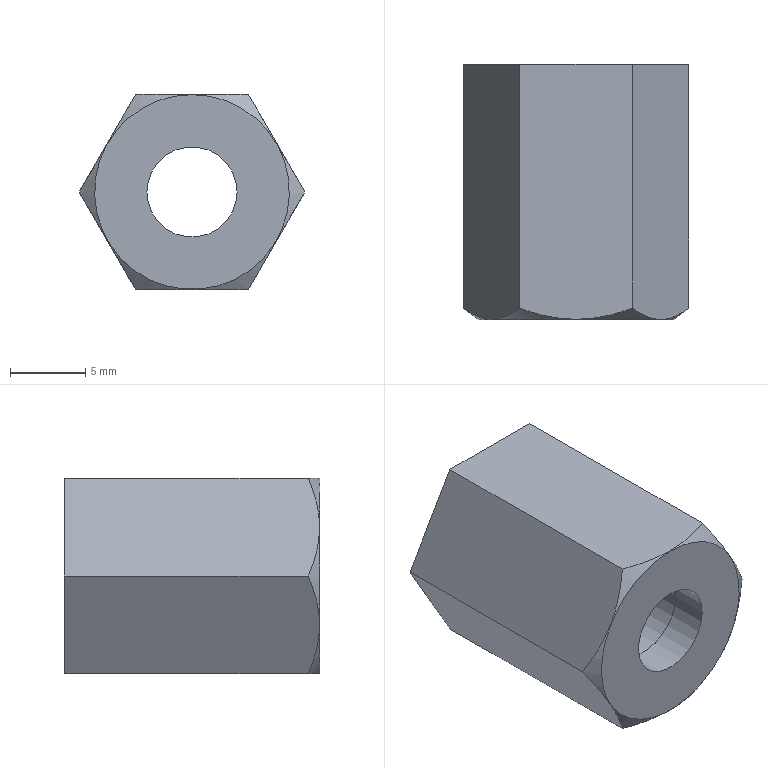Part | STEP file | 1-61.1 | 2 solids | 16 faces | box 15.011 x 17 x 13 mm | volume 1376 mm3 | plane 11 | cylinder 4 | cone 1 | commonest cylinder face diameters 6 x2 10 x2
STEP:
#1=CARTESIAN_POINT('',(0.,0.,0.));
#2=DIRECTION('',(0.,0.,1.));
#3=DIRECTION('',(1.,0.,0.));
#4=AXIS2_PLACEMENT_3D('',#1,#2,#3);
#5=CARTESIAN_POINT('',(-3.753,0.,6.5));
#6=VERTEX_POINT('',#5);
#7=CARTESIAN_POINT('',(3.753,0.,6.5));
#8=VERTEX_POINT('',#7);
#9=CARTESIAN_POINT('',(-3.753,0.,6.5));
#10=DIRECTION('',(1.,0.,0.));
#11=VECTOR('',#10,1.);
#12=LINE('',#9,#11);
#13=CARTESIAN_POINT('',(0.,0.,-1.006));
#14=DIRECTION('',(0.,1.,0.));
#15=DIRECTION('',(1.,0.,0.));
#16=AXIS2_PLACEMENT_3D('',#13,#14,#15);
#17=PLANE('',#16);
#18=CARTESIAN_POINT('',(-3.753,-7.506));
#19=DIRECTION('',(1.,0.));
#20=VECTOR('',#19,1.);
#21=LINE('',#18,#20);
#22=(GEOMETRIC_REPRESENTATION_CONTEXT(2)PARAMETRIC_REPRESENTATION_CONTEXT()REPRESENTATION_CONTEXT('',''));
#23=DEFINITIONAL_REPRESENTATION('',(#21),#22);
#24=PCURVE('',#17,#23);
#25=CARTESIAN_POINT('',(0.,-8.5,6.5));
#26=DIRECTION('',(0.,0.,-1.));
#27=DIRECTION('',(1.,0.,0.));
#28=AXIS2_PLACEMENT_3D('',#25,#26,#27);
#29=PLANE('',#28);
#30=CARTESIAN_POINT('',(-3.753,-8.5));
#31=DIRECTION('',(1.,0.));
#32=VECTOR('',#31,1.);
#33=LINE('',#30,#32);
#34=(GEOMETRIC_REPRESENTATION_CONTEXT(2)PARAMETRIC_REPRESENTATION_CONTEXT()REPRESENTATION_CONTEXT('',''));
#35=DEFINITIONAL_REPRESENTATION('',(#33),#34);
#36=PCURVE('',#29,#35);
#37=SURFACE_CURVE('',#12,(#24,#36),.PCURVE_S1.);
#38=EDGE_CURVE('',#6,#8,#37,.T.);
#39=ORIENTED_EDGE('',*,*,#38,.T.);
#40=CARTESIAN_POINT('',(7.506,0.,0.));
#41=VERTEX_POINT('',#40);
#42=CARTESIAN_POINT('',(3.753,0.,6.5));
#43=DIRECTION('',(0.5,0.,-0.866));
#44=VECTOR('',#43,1.);
#45=LINE('',#42,#44);
#46=CARTESIAN_POINT('',(3.753,-7.506));
#47=DIRECTION('',(0.5,0.866));
#48=VECTOR('',#47,1.);
#49=LINE('',#46,#48);
#50=(GEOMETRIC_REPRESENTATION_CONTEXT(2)PARAMETRIC_REPRESENTATION_CONTEXT()REPRESENTATION_CONTEXT('',''));
#51=DEFINITIONAL_REPRESENTATION('',(#49),#50);
#52=PCURVE('',#17,#51);
#53=CARTESIAN_POINT('',(5.629,-8.5,3.25));
#54=DIRECTION('',(-0.866,0.,-0.5));
#55=DIRECTION('',(0.5,0.,-0.866));
#56=AXIS2_PLACEMENT_3D('',#53,#54,#55);
#57=PLANE('',#56);
#58=CARTESIAN_POINT('',(-3.753,-8.5));
#59=DIRECTION('',(1.,0.));
#60=VECTOR('',#59,1.);
#61=LINE('',#58,#60);
#62=(GEOMETRIC_REPRESENTATION_CONTEXT(2)PARAMETRIC_REPRESENTATION_CONTEXT()REPRESENTATION_CONTEXT('',''));
#63=DEFINITIONAL_REPRESENTATION('',(#61),#62);
#64=PCURVE('',#57,#63);
#65=SURFACE_CURVE('',#45,(#52,#64),.PCURVE_S1.);
#66=EDGE_CURVE('',#8,#41,#65,.T.);
#67=ORIENTED_EDGE('',*,*,#66,.T.);
#68=CARTESIAN_POINT('',(3.753,0.,-6.5));
#69=VERTEX_POINT('',#68);
#70=CARTESIAN_POINT('',(7.506,0.,0.));
#71=DIRECTION('',(-0.5,0.,-0.866));
#72=VECTOR('',#71,1.);
#73=LINE('',#70,#72);
#74=CARTESIAN_POINT('',(7.506,-1.006));
#75=DIRECTION('',(-0.5,0.866));
#76=VECTOR('',#75,1.);
#77=LINE('',#74,#76);
#78=(GEOMETRIC_REPRESENTATION_CONTEXT(2)PARAMETRIC_REPRESENTATION_CONTEXT()REPRESENTATION_CONTEXT('',''));
#79=DEFINITIONAL_REPRESENTATION('',(#77),#78);
#80=PCURVE('',#17,#79);
#81=CARTESIAN_POINT('',(5.629,-8.5,-3.25));
#82=DIRECTION('',(-0.866,0.,0.5));
#83=DIRECTION('',(-0.5,0.,-0.866));
#84=AXIS2_PLACEMENT_3D('',#81,#82,#83);
#85=PLANE('',#84);
#86=CARTESIAN_POINT('',(-3.753,-8.5));
#87=DIRECTION('',(1.,0.));
#88=VECTOR('',#87,1.);
#89=LINE('',#86,#88);
#90=(GEOMETRIC_REPRESENTATION_CONTEXT(2)PARAMETRIC_REPRESENTATION_CONTEXT()REPRESENTATION_CONTEXT('',''));
#91=DEFINITIONAL_REPRESENTATION('',(#89),#90);
#92=PCURVE('',#85,#91);
#93=SURFACE_CURVE('',#73,(#80,#92),.PCURVE_S1.);
#94=EDGE_CURVE('',#41,#69,#93,.T.);
#95=ORIENTED_EDGE('',*,*,#94,.T.);
#96=CARTESIAN_POINT('',(-3.753,0.,-6.5));
#97=VERTEX_POINT('',#96);
#98=CARTESIAN_POINT('',(3.753,0.,-6.5));
#99=DIRECTION('',(-1.,0.,0.));
#100=VECTOR('',#99,1.);
#101=LINE('',#98,#100);
#102=CARTESIAN_POINT('',(3.753,5.494));
#103=DIRECTION('',(-1.,0.));
#104=VECTOR('',#103,1.);
#105=LINE('',#102,#104);
#106=(GEOMETRIC_REPRESENTATION_CONTEXT(2)PARAMETRIC_REPRESENTATION_CONTEXT()REPRESENTATION_CONTEXT('',''));
#107=DEFINITIONAL_REPRESENTATION('',(#105),#106);
#108=PCURVE('',#17,#107);
#109=CARTESIAN_POINT('',(0.,-8.5,-6.5));
#110=DIRECTION('',(0.,0.,1.));
#111=DIRECTION('',(-1.,0.,0.));
#112=AXIS2_PLACEMENT_3D('',#109,#110,#111);
#113=PLANE('',#112);
#114=CARTESIAN_POINT('',(-3.753,-8.5));
#115=DIRECTION('',(1.,0.));
#116=VECTOR('',#115,1.);
#117=LINE('',#114,#116);
#118=(GEOMETRIC_REPRESENTATION_CONTEXT(2)PARAMETRIC_REPRESENTATION_CONTEXT()REPRESENTATION_CONTEXT('',''));
#119=DEFINITIONAL_REPRESENTATION('',(#117),#118);
#120=PCURVE('',#113,#119);
#121=SURFACE_CURVE('',#101,(#108,#120),.PCURVE_S1.);
#122=EDGE_CURVE('',#69,#97,#121,.T.);
#123=ORIENTED_EDGE('',*,*,#122,.T.);
#124=CARTESIAN_POINT('',(-7.506,0.,0.));
#125=VERTEX_POINT('',#124);
#126=CARTESIAN_POINT('',(-3.753,0.,-6.5));
#127=DIRECTION('',(-0.5,0.,0.866));
#128=VECTOR('',#127,1.);
#129=LINE('',#126,#128);
#130=CARTESIAN_POINT('',(-3.753,5.494));
#131=DIRECTION('',(-0.5,-0.866));
#132=VECTOR('',#131,1.);
#133=LINE('',#130,#132);
#134=(GEOMETRIC_REPRESENTATION_CONTEXT(2)PARAMETRIC_REPRESENTATION_CONTEXT()REPRESENTATION_CONTEXT('',''));
#135=DEFINITIONAL_REPRESENTATION('',(#133),#134);
#136=PCURVE('',#17,#135);
#137=CARTESIAN_POINT('',(-5.629,-8.5,-3.25));
#138=DIRECTION('',(0.866,0.,0.5));
#139=DIRECTION('',(-0.5,0.,0.866));
#140=AXIS2_PLACEMENT_3D('',#137,#138,#139);
#141=PLANE('',#140);
#142=CARTESIAN_POINT('',(-3.753,-8.5));
#143=DIRECTION('',(1.,0.));
#144=VECTOR('',#143,1.);
#145=LINE('',#142,#144);
#146=(GEOMETRIC_REPRESENTATION_CONTEXT(2)PARAMETRIC_REPRESENTATION_CONTEXT()REPRESENTATION_CONTEXT('',''));
#147=DEFINITIONAL_REPRESENTATION('',(#145),#146);
#148=PCURVE('',#141,#147);
#149=SURFACE_CURVE('',#129,(#136,#148),.PCURVE_S1.);
#150=EDGE_CURVE('',#97,#125,#149,.T.);
#151=ORIENTED_EDGE('',*,*,#150,.T.);
#152=CARTESIAN_POINT('',(-7.506,0.,0.));
#153=DIRECTION('',(0.5,0.,0.866));
#154=VECTOR('',#153,1.);
#155=LINE('',#152,#154);
#156=CARTESIAN_POINT('',(-7.506,-1.006));
#157=DIRECTION('',(0.5,-0.866));
#158=VECTOR('',#157,1.);
#159=LINE('',#156,#158);
#160=(GEOMETRIC_REPRESENTATION_CONTEXT(2)PARAMETRIC_REPRESENTATION_CONTEXT()REPRESENTATION_CONTEXT('',''));
#161=DEFINITIONAL_REPRESENTATION('',(#159),#160);
#162=PCURVE('',#17,#161);
#163=CARTESIAN_POINT('',(-5.629,-8.5,3.25));
#164=DIRECTION('',(0.866,0.,-0.5));
#165=DIRECTION('',(0.5,0.,0.866));
#166=AXIS2_PLACEMENT_3D('',#163,#164,#165);
#167=PLANE('',#166);
#168=CARTESIAN_POINT('',(-3.753,-8.5));
#169=DIRECTION('',(1.,0.));
#170=VECTOR('',#169,1.);
#171=LINE('',#168,#170);
#172=(GEOMETRIC_REPRESENTATION_CONTEXT(2)PARAMETRIC_REPRESENTATION_CONTEXT()REPRESENTATION_CONTEXT('',''));
#173=DEFINITIONAL_REPRESENTATION('',(#171),#172);
#174=PCURVE('',#167,#173);
#175=SURFACE_CURVE('',#155,(#162,#174),.PCURVE_S1.);
#176=EDGE_CURVE('',#125,#6,#175,.T.);
#177=ORIENTED_EDGE('',*,*,#176,.T.);
#178=EDGE_LOOP('',(#39,#67,#95,#123,#151,#177));
#179=FACE_BOUND('',#178,.T.);
#180=CARTESIAN_POINT('',(5.,0.,0.));
#181=VERTEX_POINT('',#180);
#182=CARTESIAN_POINT('',(0.,0.,0.));
#183=DIRECTION('',(0.,-1.,0.));
#184=DIRECTION('',(1.,0.,0.));
#185=AXIS2_PLACEMENT_3D('',#182,#183,#184);
#186=CIRCLE('',#185,5.);
#187=CARTESIAN_POINT('',(5.,-1.006));
#188=CARTESIAN_POINT('',(5.,-9.666));
#189=CARTESIAN_POINT('',(-2.5,-5.336));
#190=CARTESIAN_POINT('',(-10.,-1.006));
#191=CARTESIAN_POINT('',(-2.5,3.325));
#192=CARTESIAN_POINT('',(5.,7.655));
#193=CARTESIAN_POINT('',(5.,-1.006));
#194=(BOUNDED_CURVE()B_SPLINE_CURVE(2,(#187,#188,#189,#190,#191,#192,#193),.UNSPECIFIED.,.T.,.F.)B_SPLINE_CURVE_WITH_KNOTS((1,2,2,2,2,1),(-2.094,0.,2.094,4.189,6.283,8.378),.UNSPECIFIED.)CURVE()GEOMETRIC_REPRESENTATION_ITEM()RATIONAL_B_SPLINE_CURVE((1.,0.5,1.,0.5,1.,0.5,1.))REPRESENTATION_ITEM(''));
#195=(GEOMETRIC_REPRESENTATION_CONTEXT(2)PARAMETRIC_REPRESENTATION_CONTEXT()REPRESENTATION_CONTEXT('',''));
#196=DEFINITIONAL_REPRESENTATION('',(#194),#195);
#197=PCURVE('',#17,#196);
#198=CARTESIAN_POINT('',(0.,0.,0.));
#199=DIRECTION('',(0.,-1.,0.));
#200=DIRECTION('',(1.,0.,0.));
#201=AXIS2_PLACEMENT_3D('',#198,#199,#200);
#202=CYLINDRICAL_SURFACE('',#201,5.);
#203=CARTESIAN_POINT('',(0.,0.));
#204=DIRECTION('',(1.,0.));
#205=VECTOR('',#204,1.);
#206=LINE('',#203,#205);
#207=(GEOMETRIC_REPRESENTATION_CONTEXT(2)PARAMETRIC_REPRESENTATION_CONTEXT()REPRESENTATION_CONTEXT('',''));
#208=DEFINITIONAL_REPRESENTATION('',(#206),#207);
#209=PCURVE('',#202,#208);
#210=SURFACE_CURVE('',#186,(#197,#209),.PCURVE_S1.);
#211=EDGE_CURVE('',#181,#181,#210,.T.);
#212=ORIENTED_EDGE('',*,*,#211,.T.);
#213=EDGE_LOOP('',(#212));
#214=FACE_BOUND('',#213,.T.);
#215=ADVANCED_FACE('',(#179,#214),#17,.T.);
#216=ORIENTED_EDGE('',*,*,#211,.T.);
#217=CARTESIAN_POINT('',(5.,-14.5,0.));
#218=VERTEX_POINT('',#217);
#219=CARTESIAN_POINT('',(5.,0.,0.));
#220=DIRECTION('',(0.,-1.,0.));
#221=VECTOR('',#220,1.);
#222=LINE('',#219,#221);
#223=CARTESIAN_POINT('',(6.283,0.));
#224=DIRECTION('',(0.,1.));
#225=VECTOR('',#224,1.);
#226=LINE('',#223,#225);
#227=(GEOMETRIC_REPRESENTATION_CONTEXT(2)PARAMETRIC_REPRESENTATION_CONTEXT()REPRESENTATION_CONTEXT('',''));
#228=DEFINITIONAL_REPRESENTATION('',(#226),#227);
#229=PCURVE('',#202,#228);
#230=CARTESIAN_POINT('',(0.,0.));
#231=DIRECTION('',(0.,1.));
#232=VECTOR('',#231,1.);
#233=LINE('',#230,#232);
#234=(GEOMETRIC_REPRESENTATION_CONTEXT(2)PARAMETRIC_REPRESENTATION_CONTEXT()REPRESENTATION_CONTEXT('',''));
#235=DEFINITIONAL_REPRESENTATION('',(#233),#234);
#236=PCURVE('',#202,#235);
#237=SEAM_CURVE('',#222,(#229,#236),.PCURVE_S1.);
#238=EDGE_CURVE('',#181,#218,#237,.T.);
#239=ORIENTED_EDGE('',*,*,#238,.T.);
#240=CARTESIAN_POINT('',(0.,-14.5,0.));
#241=DIRECTION('',(0.,-1.,0.));
#242=DIRECTION('',(1.,0.,0.));
#243=AXIS2_PLACEMENT_3D('',#240,#241,#242);
#244=CIRCLE('',#243,5.);
#245=CARTESIAN_POINT('',(0.,14.5));
#246=DIRECTION('',(1.,0.));
#247=VECTOR('',#246,1.);
#248=LINE('',#245,#247);
#249=(GEOMETRIC_REPRESENTATION_CONTEXT(2)PARAMETRIC_REPRESENTATION_CONTEXT()REPRESENTATION_CONTEXT('',''));
#250=DEFINITIONAL_REPRESENTATION('',(#248),#249);
#251=PCURVE('',#202,#250);
#252=CARTESIAN_POINT('',(-1.34,-14.5,0.));
#253=DIRECTION('',(0.,-1.,0.));
#254=DIRECTION('',(1.,0.,0.));
#255=AXIS2_PLACEMENT_3D('',#252,#253,#254);
#256=PLANE('',#255);
#257=CARTESIAN_POINT('',(1.34,0.));
#258=DIRECTION('',(1.,0.));
#259=AXIS2_PLACEMENT_2D('',#257,#258);
#260=CIRCLE('',#259,5.);
#261=(GEOMETRIC_REPRESENTATION_CONTEXT(2)PARAMETRIC_REPRESENTATION_CONTEXT()REPRESENTATION_CONTEXT('',''));
#262=DEFINITIONAL_REPRESENTATION('',(#260),#261);
#263=PCURVE('',#256,#262);
#264=SURFACE_CURVE('',#244,(#251,#263),.PCURVE_S1.);
#265=EDGE_CURVE('',#218,#218,#264,.T.);
#266=ORIENTED_EDGE('',*,*,#265,.F.);
#267=ORIENTED_EDGE('',*,*,#238,.F.);
#268=EDGE_LOOP('',(#216,#239,#266,#267));
#269=FACE_BOUND('',#268,.F.);
#270=ADVANCED_FACE('',(#269),#202,.F.);
#271=ORIENTED_EDGE('',*,*,#38,.T.);
#272=CARTESIAN_POINT('',(3.753,-16.239,6.5));
#273=VERTEX_POINT('',#272);
#274=CARTESIAN_POINT('',(3.753,0.,6.5));
#275=DIRECTION('',(0.,-1.,0.));
#276=VECTOR('',#275,1.);
#277=LINE('',#274,#276);
#278=CARTESIAN_POINT('',(3.753,-8.5));
#279=DIRECTION('',(0.,1.));
#280=VECTOR('',#279,1.);
#281=LINE('',#278,#280);
#282=(GEOMETRIC_REPRESENTATION_CONTEXT(2)PARAMETRIC_REPRESENTATION_CONTEXT()REPRESENTATION_CONTEXT('',''));
#283=DEFINITIONAL_REPRESENTATION('',(#281),#282);
#284=PCURVE('',#29,#283);
#285=CARTESIAN_POINT('',(-3.753,-8.5));
#286=DIRECTION('',(0.,1.));
#287=VECTOR('',#286,1.);
#288=LINE('',#285,#287);
#289=(GEOMETRIC_REPRESENTATION_CONTEXT(2)PARAMETRIC_REPRESENTATION_CONTEXT()REPRESENTATION_CONTEXT('',''));
#290=DEFINITIONAL_REPRESENTATION('',(#288),#289);
#291=PCURVE('',#57,#290);
#292=SURFACE_CURVE('',#277,(#284,#291),.PCURVE_S1.);
#293=EDGE_CURVE('',#8,#273,#292,.T.);
#294=ORIENTED_EDGE('',*,*,#293,.T.);
#295=CARTESIAN_POINT('',(0.,-16.985,6.5));
#296=VERTEX_POINT('',#295);
#297=CARTESIAN_POINT('',(3.753,-16.239,6.5));
#298=CARTESIAN_POINT('',(1.742,-16.985,6.5));
#299=CARTESIAN_POINT('',(0.,-16.985,6.5));
#300=(BOUNDED_CURVE()B_SPLINE_CURVE(2,(#297,#298,#299),.UNSPECIFIED.,.F.,.F.)B_SPLINE_CURVE_WITH_KNOTS((3,3),(0.,1.),.PIECEWISE_BEZIER_KNOTS.)CURVE()GEOMETRIC_REPRESENTATION_ITEM()RATIONAL_B_SPLINE_CURVE((1.557,1.677,1.677))REPRESENTATION_ITEM(''));
#301=CARTESIAN_POINT('',(3.753,7.739));
#302=CARTESIAN_POINT('',(1.742,8.485));
#303=CARTESIAN_POINT('',(0.,8.485));
#304=(BOUNDED_CURVE()B_SPLINE_CURVE(2,(#301,#302,#303),.UNSPECIFIED.,.F.,.F.)B_SPLINE_CURVE_WITH_KNOTS((3,3),(0.,1.),.PIECEWISE_BEZIER_KNOTS.)CURVE()GEOMETRIC_REPRESENTATION_ITEM()RATIONAL_B_SPLINE_CURVE((1.557,1.677,1.677))REPRESENTATION_ITEM(''));
#305=(GEOMETRIC_REPRESENTATION_CONTEXT(2)PARAMETRIC_REPRESENTATION_CONTEXT()REPRESENTATION_CONTEXT('',''));
#306=DEFINITIONAL_REPRESENTATION('',(#304),#305);
#307=PCURVE('',#29,#306);
#308=CARTESIAN_POINT('',(0.,-17.,0.));
#309=DIRECTION('',(0.,1.,0.));
#310=DIRECTION('',(0.,0.,1.));
#311=AXIS2_PLACEMENT_3D('',#308,#309,#310);
#312=CONICAL_SURFACE('',#311,6.48,0.9323);
#313=CARTESIAN_POINT('',(0.5236,0.7608));
#314=CARTESIAN_POINT('',(0.516,0.7365));
#315=CARTESIAN_POINT('',(0.5008,0.6892));
#316=CARTESIAN_POINT('',(0.4779,0.6225));
#317=CARTESIAN_POINT('',(0.4548,0.5598));
#318=CARTESIAN_POINT('',(0.4317,0.501));
#319=CARTESIAN_POINT('',(0.4084,0.4461));
#320=CARTESIAN_POINT('',(0.3849,0.3948));
#321=CARTESIAN_POINT('',(0.3614,0.3471));
#322=CARTESIAN_POINT('',(0.3378,0.3029));
#323=CARTESIAN_POINT('',(0.3141,0.2621));
#324=CARTESIAN_POINT('',(0.2903,0.2246));
#325=CARTESIAN_POINT('',(0.2664,0.1903));
#326=CARTESIAN_POINT('',(0.2424,0.1593));
#327=CARTESIAN_POINT('',(0.2184,0.1314));
#328=CARTESIAN_POINT('',(0.1943,0.1065));
#329=CARTESIAN_POINT('',(0.1701,0.08468));
#330=CARTESIAN_POINT('',(0.1459,0.06585));
#331=CARTESIAN_POINT('',(0.1217,0.04996));
#332=CARTESIAN_POINT('',(0.09736,0.03701));
#333=CARTESIAN_POINT('',(0.07305,0.02696));
#334=CARTESIAN_POINT('',(0.04871,0.01979));
#335=CARTESIAN_POINT('',(0.02436,0.01549));
#336=CARTESIAN_POINT('',(0.00812,0.01454));
#337=CARTESIAN_POINT('',(0.,0.01454));
#338=B_SPLINE_CURVE_WITH_KNOTS('',3,(#313,#314,#315,#316,#317,#318,#319,#320,#321,#322,#323,#324,#325,#326,#327,#328,#329,#330,#331,#332,#333,#334,#335,#336,#337),.UNSPECIFIED.,.F.,.F.,(4,1,1,1,1,1,1,1,1,1,1,1,1,1,1,1,1,1,1,1,1,1,4),(0.,0.04545,0.09091,0.1364,0.1818,0.2273,0.2727,0.3182,0.3636,0.4091,0.4545,0.5,0.5455,0.5909,0.6364,0.6818,0.7273,0.7727,0.8182,0.8636,0.9091,0.9545,1.),.QUASI_UNIFORM_KNOTS.);
#339=(GEOMETRIC_REPRESENTATION_CONTEXT(2)PARAMETRIC_REPRESENTATION_CONTEXT()REPRESENTATION_CONTEXT('',''));
#340=DEFINITIONAL_REPRESENTATION('',(#338),#339);
#341=PCURVE('',#312,#340);
#342=SURFACE_CURVE('',#300,(#307,#341),.PCURVE_S1.);
#343=EDGE_CURVE('',#273,#296,#342,.T.);
#344=ORIENTED_EDGE('',*,*,#343,.T.);
#345=CARTESIAN_POINT('',(-3.753,-16.239,6.5));
#346=VERTEX_POINT('',#345);
#347=CARTESIAN_POINT('',(0.,-16.985,6.5));
#348=CARTESIAN_POINT('',(-1.742,-16.985,6.5));
#349=CARTESIAN_POINT('',(-3.753,-16.239,6.5));
#350=(BOUNDED_CURVE()B_SPLINE_CURVE(2,(#347,#348,#349),.UNSPECIFIED.,.F.,.F.)B_SPLINE_CURVE_WITH_KNOTS((3,3),(0.,1.),.PIECEWISE_BEZIER_KNOTS.)CURVE()GEOMETRIC_REPRESENTATION_ITEM()RATIONAL_B_SPLINE_CURVE((1.677,1.677,1.557))REPRESENTATION_ITEM(''));
#351=CARTESIAN_POINT('',(0.,8.485));
#352=CARTESIAN_POINT('',(-1.742,8.485));
#353=CARTESIAN_POINT('',(-3.753,7.739));
#354=(BOUNDED_CURVE()B_SPLINE_CURVE(2,(#351,#352,#353),.UNSPECIFIED.,.F.,.F.)B_SPLINE_CURVE_WITH_KNOTS((3,3),(0.,1.),.PIECEWISE_BEZIER_KNOTS.)CURVE()GEOMETRIC_REPRESENTATION_ITEM()RATIONAL_B_SPLINE_CURVE((1.677,1.677,1.557))REPRESENTATION_ITEM(''));
#355=(GEOMETRIC_REPRESENTATION_CONTEXT(2)PARAMETRIC_REPRESENTATION_CONTEXT()REPRESENTATION_CONTEXT('',''));
#356=DEFINITIONAL_REPRESENTATION('',(#354),#355);
#357=PCURVE('',#29,#356);
#358=CARTESIAN_POINT('',(6.283,0.01454));
#359=CARTESIAN_POINT('',(6.275,0.01454));
#360=CARTESIAN_POINT('',(6.259,0.01549));
#361=CARTESIAN_POINT('',(6.234,0.01979));
#362=CARTESIAN_POINT('',(6.21,0.02696));
#363=CARTESIAN_POINT('',(6.186,0.03701));
#364=CARTESIAN_POINT('',(6.162,0.04996));
#365=CARTESIAN_POINT('',(6.137,0.06585));
#366=CARTESIAN_POINT('',(6.113,0.08468));
#367=CARTESIAN_POINT('',(6.089,0.1065));
#368=CARTESIAN_POINT('',(6.065,0.1314));
#369=CARTESIAN_POINT('',(6.041,0.1593));
#370=CARTESIAN_POINT('',(6.017,0.1903));
#371=CARTESIAN_POINT('',(5.993,0.2246));
#372=CARTESIAN_POINT('',(5.969,0.2621));
#373=CARTESIAN_POINT('',(5.945,0.3029));
#374=CARTESIAN_POINT('',(5.922,0.3471));
#375=CARTESIAN_POINT('',(5.898,0.3948));
#376=CARTESIAN_POINT('',(5.875,0.4461));
#377=CARTESIAN_POINT('',(5.852,0.501));
#378=CARTESIAN_POINT('',(5.828,0.5598));
#379=CARTESIAN_POINT('',(5.805,0.6225));
#380=CARTESIAN_POINT('',(5.782,0.6892));
#381=CARTESIAN_POINT('',(5.767,0.7365));
#382=CARTESIAN_POINT('',(5.76,0.7608));
#383=B_SPLINE_CURVE_WITH_KNOTS('',3,(#358,#359,#360,#361,#362,#363,#364,#365,#366,#367,#368,#369,#370,#371,#372,#373,#374,#375,#376,#377,#378,#379,#380,#381,#382),.UNSPECIFIED.,.F.,.F.,(4,1,1,1,1,1,1,1,1,1,1,1,1,1,1,1,1,1,1,1,1,1,4),(0.,0.04545,0.09091,0.1364,0.1818,0.2273,0.2727,0.3182,0.3636,0.4091,0.4545,0.5,0.5455,0.5909,0.6364,0.6818,0.7273,0.7727,0.8182,0.8636,0.9091,0.9545,1.),.QUASI_UNIFORM_KNOTS.);
#384=(GEOMETRIC_REPRESENTATION_CONTEXT(2)PARAMETRIC_REPRESENTATION_CONTEXT()REPRESENTATION_CONTEXT('',''));
#385=DEFINITIONAL_REPRESENTATION('',(#383),#384);
#386=PCURVE('',#312,#385);
#387=SURFACE_CURVE('',#350,(#357,#386),.PCURVE_S1.);
#388=EDGE_CURVE('',#296,#346,#387,.T.);
#389=ORIENTED_EDGE('',*,*,#388,.T.);
#390=CARTESIAN_POINT('',(-3.753,0.,6.5));
#391=DIRECTION('',(0.,-1.,0.));
#392=VECTOR('',#391,1.);
#393=LINE('',#390,#392);
#394=CARTESIAN_POINT('',(-3.753,-8.5));
#395=DIRECTION('',(0.,1.));
#396=VECTOR('',#395,1.);
#397=LINE('',#394,#396);
#398=(GEOMETRIC_REPRESENTATION_CONTEXT(2)PARAMETRIC_REPRESENTATION_CONTEXT()REPRESENTATION_CONTEXT('',''));
#399=DEFINITIONAL_REPRESENTATION('',(#397),#398);
#400=PCURVE('',#29,#399);
#401=CARTESIAN_POINT('',(3.753,-8.5));
#402=DIRECTION('',(0.,1.));
#403=VECTOR('',#402,1.);
#404=LINE('',#401,#403);
#405=(GEOMETRIC_REPRESENTATION_CONTEXT(2)PARAMETRIC_REPRESENTATION_CONTEXT()REPRESENTATION_CONTEXT('',''));
#406=DEFINITIONAL_REPRESENTATION('',(#404),#405);
#407=PCURVE('',#167,#406);
#408=SURFACE_CURVE('',#393,(#400,#407),.PCURVE_S1.);
#409=EDGE_CURVE('',#6,#346,#408,.T.);
#410=ORIENTED_EDGE('',*,*,#409,.F.);
#411=EDGE_LOOP('',(#271,#294,#344,#389,#410));
#412=FACE_BOUND('',#411,.F.);
#413=ADVANCED_FACE('',(#412),#29,.F.);
#414=ORIENTED_EDGE('',*,*,#66,.T.);
#415=CARTESIAN_POINT('',(7.506,-16.239,0.));
#416=VERTEX_POINT('',#415);
#417=CARTESIAN_POINT('',(7.506,0.,0.));
#418=DIRECTION('',(0.,-1.,0.));
#419=VECTOR('',#418,1.);
#420=LINE('',#417,#419);
#421=CARTESIAN_POINT('',(3.753,-8.5));
#422=DIRECTION('',(0.,1.));
#423=VECTOR('',#422,1.);
#424=LINE('',#421,#423);
#425=(GEOMETRIC_REPRESENTATION_CONTEXT(2)PARAMETRIC_REPRESENTATION_CONTEXT()REPRESENTATION_CONTEXT('',''));
#426=DEFINITIONAL_REPRESENTATION('',(#424),#425);
#427=PCURVE('',#57,#426);
#428=CARTESIAN_POINT('',(-3.753,-8.5));
#429=DIRECTION('',(0.,1.));
#430=VECTOR('',#429,1.);
#431=LINE('',#428,#430);
#432=(GEOMETRIC_REPRESENTATION_CONTEXT(2)PARAMETRIC_REPRESENTATION_CONTEXT()REPRESENTATION_CONTEXT('',''));
#433=DEFINITIONAL_REPRESENTATION('',(#431),#432);
#434=PCURVE('',#85,#433);
#435=SURFACE_CURVE('',#420,(#427,#434),.PCURVE_S1.);
#436=EDGE_CURVE('',#41,#416,#435,.T.);
#437=ORIENTED_EDGE('',*,*,#436,.T.);
#438=CARTESIAN_POINT('',(7.506,-16.239,0.));
#439=CARTESIAN_POINT('',(5.629,-17.632,3.25));
#440=CARTESIAN_POINT('',(3.753,-16.239,6.5));
#441=(BOUNDED_CURVE()B_SPLINE_CURVE(2,(#438,#439,#440),.UNSPECIFIED.,.F.,.F.)B_SPLINE_CURVE_WITH_KNOTS((3,3),(0.,1.),.PIECEWISE_BEZIER_KNOTS.)CURVE()GEOMETRIC_REPRESENTATION_ITEM()RATIONAL_B_SPLINE_CURVE((1.557,1.797,1.557))REPRESENTATION_ITEM(''));
#442=CARTESIAN_POINT('',(3.753,7.739));
#443=CARTESIAN_POINT('',(0.,9.132));
#444=CARTESIAN_POINT('',(-3.753,7.739));
#445=(BOUNDED_CURVE()B_SPLINE_CURVE(2,(#442,#443,#444),.UNSPECIFIED.,.F.,.F.)B_SPLINE_CURVE_WITH_KNOTS((3,3),(0.,1.),.PIECEWISE_BEZIER_KNOTS.)CURVE()GEOMETRIC_REPRESENTATION_ITEM()RATIONAL_B_SPLINE_CURVE((1.557,1.797,1.557))REPRESENTATION_ITEM(''));
#446=(GEOMETRIC_REPRESENTATION_CONTEXT(2)PARAMETRIC_REPRESENTATION_CONTEXT()REPRESENTATION_CONTEXT('',''));
#447=DEFINITIONAL_REPRESENTATION('',(#445),#446);
#448=PCURVE('',#57,#447);
#449=CARTESIAN_POINT('',(1.571,0.7608));
#450=CARTESIAN_POINT('',(1.556,0.7121));
#451=CARTESIAN_POINT('',(1.525,0.6204));
#452=CARTESIAN_POINT('',(1.479,0.4991));
#453=CARTESIAN_POINT('',(1.432,0.393));
#454=CARTESIAN_POINT('',(1.385,0.3012));
#455=CARTESIAN_POINT('',(1.338,0.223));
#456=CARTESIAN_POINT('',(1.29,0.1577));
#457=CARTESIAN_POINT('',(1.241,0.105));
#458=CARTESIAN_POINT('',(1.193,0.06437));
#459=CARTESIAN_POINT('',(1.145,0.03556));
#460=CARTESIAN_POINT('',(1.096,0.01835));
#461=CARTESIAN_POINT('',(1.047,0.01263));
#462=CARTESIAN_POINT('',(0.9985,0.01835));
#463=CARTESIAN_POINT('',(0.9498,0.03556));
#464=CARTESIAN_POINT('',(0.9013,0.06437));
#465=CARTESIAN_POINT('',(0.8529,0.105));
#466=CARTESIAN_POINT('',(0.8048,0.1577));
#467=CARTESIAN_POINT('',(0.7569,0.223));
#468=CARTESIAN_POINT('',(0.7094,0.3012));
#469=CARTESIAN_POINT('',(0.6622,0.393));
#470=CARTESIAN_POINT('',(0.6155,0.4991));
#471=CARTESIAN_POINT('',(0.5692,0.6204));
#472=CARTESIAN_POINT('',(0.5388,0.7121));
#473=CARTESIAN_POINT('',(0.5236,0.7608));
#474=B_SPLINE_CURVE_WITH_KNOTS('',3,(#449,#450,#451,#452,#453,#454,#455,#456,#457,#458,#459,#460,#461,#462,#463,#464,#465,#466,#467,#468,#469,#470,#471,#472,#473),.UNSPECIFIED.,.F.,.F.,(4,1,1,1,1,1,1,1,1,1,1,1,1,1,1,1,1,1,1,1,1,1,4),(0.,0.04545,0.09091,0.1364,0.1818,0.2273,0.2727,0.3182,0.3636,0.4091,0.4545,0.5,0.5455,0.5909,0.6364,0.6818,0.7273,0.7727,0.8182,0.8636,0.9091,0.9545,1.),.QUASI_UNIFORM_KNOTS.);
#475=(GEOMETRIC_REPRESENTATION_CONTEXT(2)PARAMETRIC_REPRESENTATION_CONTEXT()REPRESENTATION_CONTEXT('',''));
#476=DEFINITIONAL_REPRESENTATION('',(#474),#475);
#477=PCURVE('',#312,#476);
#478=SURFACE_CURVE('',#441,(#448,#477),.PCURVE_S1.);
#479=EDGE_CURVE('',#416,#273,#478,.T.);
#480=ORIENTED_EDGE('',*,*,#479,.T.);
#481=ORIENTED_EDGE('',*,*,#293,.F.);
#482=EDGE_LOOP('',(#414,#437,#480,#481));
#483=FACE_BOUND('',#482,.F.);
#484=ADVANCED_FACE('',(#483),#57,.F.);
#485=ORIENTED_EDGE('',*,*,#94,.T.);
#486=CARTESIAN_POINT('',(3.753,-16.239,-6.5));
#487=VERTEX_POINT('',#486);
#488=CARTESIAN_POINT('',(3.753,0.,-6.5));
#489=DIRECTION('',(0.,-1.,0.));
#490=VECTOR('',#489,1.);
#491=LINE('',#488,#490);
#492=CARTESIAN_POINT('',(3.753,-8.5));
#493=DIRECTION('',(0.,1.));
#494=VECTOR('',#493,1.);
#495=LINE('',#492,#494);
#496=(GEOMETRIC_REPRESENTATION_CONTEXT(2)PARAMETRIC_REPRESENTATION_CONTEXT()REPRESENTATION_CONTEXT('',''));
#497=DEFINITIONAL_REPRESENTATION('',(#495),#496);
#498=PCURVE('',#85,#497);
#499=CARTESIAN_POINT('',(-3.753,-8.5));
#500=DIRECTION('',(0.,1.));
#501=VECTOR('',#500,1.);
#502=LINE('',#499,#501);
#503=(GEOMETRIC_REPRESENTATION_CONTEXT(2)PARAMETRIC_REPRESENTATION_CONTEXT()REPRESENTATION_CONTEXT('',''));
#504=DEFINITIONAL_REPRESENTATION('',(#502),#503);
#505=PCURVE('',#113,#504);
#506=SURFACE_CURVE('',#491,(#498,#505),.PCURVE_S1.);
#507=EDGE_CURVE('',#69,#487,#506,.T.);
#508=ORIENTED_EDGE('',*,*,#507,.T.);
#509=CARTESIAN_POINT('',(3.753,-16.239,-6.5));
#510=CARTESIAN_POINT('',(5.629,-17.632,-3.25));
#511=CARTESIAN_POINT('',(7.506,-16.239,0.));
#512=(BOUNDED_CURVE()B_SPLINE_CURVE(2,(#509,#510,#511),.UNSPECIFIED.,.F.,.F.)B_SPLINE_CURVE_WITH_KNOTS((3,3),(0.,1.),.PIECEWISE_BEZIER_KNOTS.)CURVE()GEOMETRIC_REPRESENTATION_ITEM()RATIONAL_B_SPLINE_CURVE((1.557,1.797,1.557))REPRESENTATION_ITEM(''));
#513=CARTESIAN_POINT('',(3.753,7.739));
#514=CARTESIAN_POINT('',(0.,9.132));
#515=CARTESIAN_POINT('',(-3.753,7.739));
#516=(BOUNDED_CURVE()B_SPLINE_CURVE(2,(#513,#514,#515),.UNSPECIFIED.,.F.,.F.)B_SPLINE_CURVE_WITH_KNOTS((3,3),(0.,1.),.PIECEWISE_BEZIER_KNOTS.)CURVE()GEOMETRIC_REPRESENTATION_ITEM()RATIONAL_B_SPLINE_CURVE((1.557,1.797,1.557))REPRESENTATION_ITEM(''));
#517=(GEOMETRIC_REPRESENTATION_CONTEXT(2)PARAMETRIC_REPRESENTATION_CONTEXT()REPRESENTATION_CONTEXT('',''));
#518=DEFINITIONAL_REPRESENTATION('',(#516),#517);
#519=PCURVE('',#85,#518);
#520=CARTESIAN_POINT('',(2.618,0.7608));
#521=CARTESIAN_POINT('',(2.603,0.7121));
#522=CARTESIAN_POINT('',(2.572,0.6204));
#523=CARTESIAN_POINT('',(2.526,0.4991));
#524=CARTESIAN_POINT('',(2.479,0.393));
#525=CARTESIAN_POINT('',(2.432,0.3012));
#526=CARTESIAN_POINT('',(2.385,0.223));
#527=CARTESIAN_POINT('',(2.337,0.1577));
#528=CARTESIAN_POINT('',(2.289,0.105));
#529=CARTESIAN_POINT('',(2.24,0.06437));
#530=CARTESIAN_POINT('',(2.192,0.03556));
#531=CARTESIAN_POINT('',(2.143,0.01835));
#532=CARTESIAN_POINT('',(2.094,0.01263));
#533=CARTESIAN_POINT('',(2.046,0.01835));
#534=CARTESIAN_POINT('',(1.997,0.03556));
#535=CARTESIAN_POINT('',(1.948,0.06437));
#536=CARTESIAN_POINT('',(1.9,0.105));
#537=CARTESIAN_POINT('',(1.852,0.1577));
#538=CARTESIAN_POINT('',(1.804,0.223));
#539=CARTESIAN_POINT('',(1.757,0.3012));
#540=CARTESIAN_POINT('',(1.709,0.393));
#541=CARTESIAN_POINT('',(1.663,0.4991));
#542=CARTESIAN_POINT('',(1.616,0.6204));
#543=CARTESIAN_POINT('',(1.586,0.7121));
#544=CARTESIAN_POINT('',(1.571,0.7608));
#545=B_SPLINE_CURVE_WITH_KNOTS('',3,(#520,#521,#522,#523,#524,#525,#526,#527,#528,#529,#530,#531,#532,#533,#534,#535,#536,#537,#538,#539,#540,#541,#542,#543,#544),.UNSPECIFIED.,.F.,.F.,(4,1,1,1,1,1,1,1,1,1,1,1,1,1,1,1,1,1,1,1,1,1,4),(0.,0.04545,0.09091,0.1364,0.1818,0.2273,0.2727,0.3182,0.3636,0.4091,0.4545,0.5,0.5455,0.5909,0.6364,0.6818,0.7273,0.7727,0.8182,0.8636,0.9091,0.9545,1.),.QUASI_UNIFORM_KNOTS.);
#546=(GEOMETRIC_REPRESENTATION_CONTEXT(2)PARAMETRIC_REPRESENTATION_CONTEXT()REPRESENTATION_CONTEXT('',''));
#547=DEFINITIONAL_REPRESENTATION('',(#545),#546);
#548=PCURVE('',#312,#547);
#549=SURFACE_CURVE('',#512,(#519,#548),.PCURVE_S1.);
#550=EDGE_CURVE('',#487,#416,#549,.T.);
#551=ORIENTED_EDGE('',*,*,#550,.T.);
#552=ORIENTED_EDGE('',*,*,#436,.F.);
#553=EDGE_LOOP('',(#485,#508,#551,#552));
#554=FACE_BOUND('',#553,.F.);
#555=ADVANCED_FACE('',(#554),#85,.F.);
#556=ORIENTED_EDGE('',*,*,#122,.T.);
#557=CARTESIAN_POINT('',(-3.753,-16.239,-6.5));
#558=VERTEX_POINT('',#557);
#559=CARTESIAN_POINT('',(-3.753,0.,-6.5));
#560=DIRECTION('',(0.,-1.,0.));
#561=VECTOR('',#560,1.);
#562=LINE('',#559,#561);
#563=CARTESIAN_POINT('',(3.753,-8.5));
#564=DIRECTION('',(0.,1.));
#565=VECTOR('',#564,1.);
#566=LINE('',#563,#565);
#567=(GEOMETRIC_REPRESENTATION_CONTEXT(2)PARAMETRIC_REPRESENTATION_CONTEXT()REPRESENTATION_CONTEXT('',''));
#568=DEFINITIONAL_REPRESENTATION('',(#566),#567);
#569=PCURVE('',#113,#568);
#570=CARTESIAN_POINT('',(-3.753,-8.5));
#571=DIRECTION('',(0.,1.));
#572=VECTOR('',#571,1.);
#573=LINE('',#570,#572);
#574=(GEOMETRIC_REPRESENTATION_CONTEXT(2)PARAMETRIC_REPRESENTATION_CONTEXT()REPRESENTATION_CONTEXT('',''));
#575=DEFINITIONAL_REPRESENTATION('',(#573),#574);
#576=PCURVE('',#141,#575);
#577=SURFACE_CURVE('',#562,(#569,#576),.PCURVE_S1.);
#578=EDGE_CURVE('',#97,#558,#577,.T.);
#579=ORIENTED_EDGE('',*,*,#578,.T.);
#580=CARTESIAN_POINT('',(-3.753,-16.239,-6.5));
#581=CARTESIAN_POINT('',(0.,-17.632,-6.5));
#582=CARTESIAN_POINT('',(3.753,-16.239,-6.5));
#583=(BOUNDED_CURVE()B_SPLINE_CURVE(2,(#580,#581,#582),.UNSPECIFIED.,.F.,.F.)B_SPLINE_CURVE_WITH_KNOTS((3,3),(0.,1.),.PIECEWISE_BEZIER_KNOTS.)CURVE()GEOMETRIC_REPRESENTATION_ITEM()RATIONAL_B_SPLINE_CURVE((1.557,1.797,1.557))REPRESENTATION_ITEM(''));
#584=CARTESIAN_POINT('',(3.753,7.739));
#585=CARTESIAN_POINT('',(0.,9.132));
#586=CARTESIAN_POINT('',(-3.753,7.739));
#587=(BOUNDED_CURVE()B_SPLINE_CURVE(2,(#584,#585,#586),.UNSPECIFIED.,.F.,.F.)B_SPLINE_CURVE_WITH_KNOTS((3,3),(0.,1.),.PIECEWISE_BEZIER_KNOTS.)CURVE()GEOMETRIC_REPRESENTATION_ITEM()RATIONAL_B_SPLINE_CURVE((1.557,1.797,1.557))REPRESENTATION_ITEM(''));
#588=(GEOMETRIC_REPRESENTATION_CONTEXT(2)PARAMETRIC_REPRESENTATION_CONTEXT()REPRESENTATION_CONTEXT('',''));
#589=DEFINITIONAL_REPRESENTATION('',(#587),#588);
#590=PCURVE('',#113,#589);
#591=CARTESIAN_POINT('',(3.665,0.7608));
#592=CARTESIAN_POINT('',(3.65,0.7121));
#593=CARTESIAN_POINT('',(3.62,0.6204));
#594=CARTESIAN_POINT('',(3.573,0.4991));
#595=CARTESIAN_POINT('',(3.527,0.393));
#596=CARTESIAN_POINT('',(3.479,0.3012));
#597=CARTESIAN_POINT('',(3.432,0.223));
#598=CARTESIAN_POINT('',(3.384,0.1577));
#599=CARTESIAN_POINT('',(3.336,0.105));
#600=CARTESIAN_POINT('',(3.288,0.06437));
#601=CARTESIAN_POINT('',(3.239,0.03556));
#602=CARTESIAN_POINT('',(3.19,0.01835));
#603=CARTESIAN_POINT('',(3.142,0.01263));
#604=CARTESIAN_POINT('',(3.093,0.01835));
#605=CARTESIAN_POINT('',(3.044,0.03556));
#606=CARTESIAN_POINT('',(2.996,0.06437));
#607=CARTESIAN_POINT('',(2.947,0.105));
#608=CARTESIAN_POINT('',(2.899,0.1577));
#609=CARTESIAN_POINT('',(2.851,0.223));
#610=CARTESIAN_POINT('',(2.804,0.3012));
#611=CARTESIAN_POINT('',(2.757,0.393));
#612=CARTESIAN_POINT('',(2.71,0.4991));
#613=CARTESIAN_POINT('',(2.664,0.6204));
#614=CARTESIAN_POINT('',(2.633,0.7121));
#615=CARTESIAN_POINT('',(2.618,0.7608));
#616=B_SPLINE_CURVE_WITH_KNOTS('',3,(#591,#592,#593,#594,#595,#596,#597,#598,#599,#600,#601,#602,#603,#604,#605,#606,#607,#608,#609,#610,#611,#612,#613,#614,#615),.UNSPECIFIED.,.F.,.F.,(4,1,1,1,1,1,1,1,1,1,1,1,1,1,1,1,1,1,1,1,1,1,4),(0.,0.04545,0.09091,0.1364,0.1818,0.2273,0.2727,0.3182,0.3636,0.4091,0.4545,0.5,0.5455,0.5909,0.6364,0.6818,0.7273,0.7727,0.8182,0.8636,0.9091,0.9545,1.),.QUASI_UNIFORM_KNOTS.);
#617=(GEOMETRIC_REPRESENTATION_CONTEXT(2)PARAMETRIC_REPRESENTATION_CONTEXT()REPRESENTATION_CONTEXT('',''));
#618=DEFINITIONAL_REPRESENTATION('',(#616),#617);
#619=PCURVE('',#312,#618);
#620=SURFACE_CURVE('',#583,(#590,#619),.PCURVE_S1.);
#621=EDGE_CURVE('',#558,#487,#620,.T.);
#622=ORIENTED_EDGE('',*,*,#621,.T.);
#623=ORIENTED_EDGE('',*,*,#507,.F.);
#624=EDGE_LOOP('',(#556,#579,#622,#623));
#625=FACE_BOUND('',#624,.F.);
#626=ADVANCED_FACE('',(#625),#113,.F.);
#627=ORIENTED_EDGE('',*,*,#150,.T.);
#628=CARTESIAN_POINT('',(-7.506,-16.239,0.));
#629=VERTEX_POINT('',#628);
#630=CARTESIAN_POINT('',(-7.506,0.,0.));
#631=DIRECTION('',(0.,-1.,0.));
#632=VECTOR('',#631,1.);
#633=LINE('',#630,#632);
#634=CARTESIAN_POINT('',(3.753,-8.5));
#635=DIRECTION('',(0.,1.));
#636=VECTOR('',#635,1.);
#637=LINE('',#634,#636);
#638=(GEOMETRIC_REPRESENTATION_CONTEXT(2)PARAMETRIC_REPRESENTATION_CONTEXT()REPRESENTATION_CONTEXT('',''));
#639=DEFINITIONAL_REPRESENTATION('',(#637),#638);
#640=PCURVE('',#141,#639);
#641=CARTESIAN_POINT('',(-3.753,-8.5));
#642=DIRECTION('',(0.,1.));
#643=VECTOR('',#642,1.);
#644=LINE('',#641,#643);
#645=(GEOMETRIC_REPRESENTATION_CONTEXT(2)PARAMETRIC_REPRESENTATION_CONTEXT()REPRESENTATION_CONTEXT('',''));
#646=DEFINITIONAL_REPRESENTATION('',(#644),#645);
#647=PCURVE('',#167,#646);
#648=SURFACE_CURVE('',#633,(#640,#647),.PCURVE_S1.);
#649=EDGE_CURVE('',#125,#629,#648,.T.);
#650=ORIENTED_EDGE('',*,*,#649,.T.);
#651=CARTESIAN_POINT('',(-7.506,-16.239,0.));
#652=CARTESIAN_POINT('',(-5.629,-17.632,-3.25));
#653=CARTESIAN_POINT('',(-3.753,-16.239,-6.5));
#654=(BOUNDED_CURVE()B_SPLINE_CURVE(2,(#651,#652,#653),.UNSPECIFIED.,.F.,.F.)B_SPLINE_CURVE_WITH_KNOTS((3,3),(0.,1.),.PIECEWISE_BEZIER_KNOTS.)CURVE()GEOMETRIC_REPRESENTATION_ITEM()RATIONAL_B_SPLINE_CURVE((1.557,1.797,1.557))REPRESENTATION_ITEM(''));
#655=CARTESIAN_POINT('',(3.753,7.739));
#656=CARTESIAN_POINT('',(0.,9.132));
#657=CARTESIAN_POINT('',(-3.753,7.739));
#658=(BOUNDED_CURVE()B_SPLINE_CURVE(2,(#655,#656,#657),.UNSPECIFIED.,.F.,.F.)B_SPLINE_CURVE_WITH_KNOTS((3,3),(0.,1.),.PIECEWISE_BEZIER_KNOTS.)CURVE()GEOMETRIC_REPRESENTATION_ITEM()RATIONAL_B_SPLINE_CURVE((1.557,1.797,1.557))REPRESENTATION_ITEM(''));
#659=(GEOMETRIC_REPRESENTATION_CONTEXT(2)PARAMETRIC_REPRESENTATION_CONTEXT()REPRESENTATION_CONTEXT('',''));
#660=DEFINITIONAL_REPRESENTATION('',(#658),#659);
#661=PCURVE('',#141,#660);
#662=CARTESIAN_POINT('',(4.712,0.7608));
#663=CARTESIAN_POINT('',(4.697,0.7121));
#664=CARTESIAN_POINT('',(4.667,0.6204));
#665=CARTESIAN_POINT('',(4.621,0.4991));
#666=CARTESIAN_POINT('',(4.574,0.393));
#667=CARTESIAN_POINT('',(4.527,0.3012));
#668=CARTESIAN_POINT('',(4.479,0.223));
#669=CARTESIAN_POINT('',(4.431,0.1577));
#670=CARTESIAN_POINT('',(4.383,0.105));
#671=CARTESIAN_POINT('',(4.335,0.06437));
#672=CARTESIAN_POINT('',(4.286,0.03556));
#673=CARTESIAN_POINT('',(4.238,0.01835));
#674=CARTESIAN_POINT('',(4.189,0.01263));
#675=CARTESIAN_POINT('',(4.14,0.01835));
#676=CARTESIAN_POINT('',(4.091,0.03556));
#677=CARTESIAN_POINT('',(4.043,0.06437));
#678=CARTESIAN_POINT('',(3.994,0.105));
#679=CARTESIAN_POINT('',(3.946,0.1577));
#680=CARTESIAN_POINT('',(3.898,0.223));
#681=CARTESIAN_POINT('',(3.851,0.3012));
#682=CARTESIAN_POINT('',(3.804,0.393));
#683=CARTESIAN_POINT('',(3.757,0.4991));
#684=CARTESIAN_POINT('',(3.711,0.6204));
#685=CARTESIAN_POINT('',(3.68,0.7121));
#686=CARTESIAN_POINT('',(3.665,0.7608));
#687=B_SPLINE_CURVE_WITH_KNOTS('',3,(#662,#663,#664,#665,#666,#667,#668,#669,#670,#671,#672,#673,#674,#675,#676,#677,#678,#679,#680,#681,#682,#683,#684,#685,#686),.UNSPECIFIED.,.F.,.F.,(4,1,1,1,1,1,1,1,1,1,1,1,1,1,1,1,1,1,1,1,1,1,4),(0.,0.04545,0.09091,0.1364,0.1818,0.2273,0.2727,0.3182,0.3636,0.4091,0.4545,0.5,0.5455,0.5909,0.6364,0.6818,0.7273,0.7727,0.8182,0.8636,0.9091,0.9545,1.),.QUASI_UNIFORM_KNOTS.);
#688=(GEOMETRIC_REPRESENTATION_CONTEXT(2)PARAMETRIC_REPRESENTATION_CONTEXT()REPRESENTATION_CONTEXT('',''));
#689=DEFINITIONAL_REPRESENTATION('',(#687),#688);
#690=PCURVE('',#312,#689);
#691=SURFACE_CURVE('',#654,(#661,#690),.PCURVE_S1.);
#692=EDGE_CURVE('',#629,#558,#691,.T.);
#693=ORIENTED_EDGE('',*,*,#692,.T.);
#694=ORIENTED_EDGE('',*,*,#578,.F.);
#695=EDGE_LOOP('',(#627,#650,#693,#694));
#696=FACE_BOUND('',#695,.F.);
#697=ADVANCED_FACE('',(#696),#141,.F.);
#698=ORIENTED_EDGE('',*,*,#176,.T.);
#699=ORIENTED_EDGE('',*,*,#409,.T.);
#700=CARTESIAN_POINT('',(-3.753,-16.239,6.5));
#701=CARTESIAN_POINT('',(-5.629,-17.632,3.25));
#702=CARTESIAN_POINT('',(-7.506,-16.239,0.));
#703=(BOUNDED_CURVE()B_SPLINE_CURVE(2,(#700,#701,#702),.UNSPECIFIED.,.F.,.F.)B_SPLINE_CURVE_WITH_KNOTS((3,3),(0.,1.),.PIECEWISE_BEZIER_KNOTS.)CURVE()GEOMETRIC_REPRESENTATION_ITEM()RATIONAL_B_SPLINE_CURVE((1.557,1.797,1.557))REPRESENTATION_ITEM(''));
#704=CARTESIAN_POINT('',(3.753,7.739));
#705=CARTESIAN_POINT('',(0.,9.132));
#706=CARTESIAN_POINT('',(-3.753,7.739));
#707=(BOUNDED_CURVE()B_SPLINE_CURVE(2,(#704,#705,#706),.UNSPECIFIED.,.F.,.F.)B_SPLINE_CURVE_WITH_KNOTS((3,3),(0.,1.),.PIECEWISE_BEZIER_KNOTS.)CURVE()GEOMETRIC_REPRESENTATION_ITEM()RATIONAL_B_SPLINE_CURVE((1.557,1.797,1.557))REPRESENTATION_ITEM(''));
#708=(GEOMETRIC_REPRESENTATION_CONTEXT(2)PARAMETRIC_REPRESENTATION_CONTEXT()REPRESENTATION_CONTEXT('',''));
#709=DEFINITIONAL_REPRESENTATION('',(#707),#708);
#710=PCURVE('',#167,#709);
#711=CARTESIAN_POINT('',(5.76,0.7608));
#712=CARTESIAN_POINT('',(5.744,0.7121));
#713=CARTESIAN_POINT('',(5.714,0.6204));
#714=CARTESIAN_POINT('',(5.668,0.4991));
#715=CARTESIAN_POINT('',(5.621,0.393));
#716=CARTESIAN_POINT('',(5.574,0.3012));
#717=CARTESIAN_POINT('',(5.526,0.223));
#718=CARTESIAN_POINT('',(5.478,0.1577));
#719=CARTESIAN_POINT('',(5.43,0.105));
#720=CARTESIAN_POINT('',(5.382,0.06437));
#721=CARTESIAN_POINT('',(5.333,0.03556));
#722=CARTESIAN_POINT('',(5.285,0.01835));
#723=CARTESIAN_POINT('',(5.236,0.01263));
#724=CARTESIAN_POINT('',(5.187,0.01835));
#725=CARTESIAN_POINT('',(5.139,0.03556));
#726=CARTESIAN_POINT('',(5.09,0.06437));
#727=CARTESIAN_POINT('',(5.042,0.105));
#728=CARTESIAN_POINT('',(4.994,0.1577));
#729=CARTESIAN_POINT('',(4.946,0.223));
#730=CARTESIAN_POINT('',(4.898,0.3012));
#731=CARTESIAN_POINT('',(4.851,0.393));
#732=CARTESIAN_POINT('',(4.804,0.4991));
#733=CARTESIAN_POINT('',(4.758,0.6204));
#734=CARTESIAN_POINT('',(4.728,0.7121));
#735=CARTESIAN_POINT('',(4.712,0.7608));
#736=B_SPLINE_CURVE_WITH_KNOTS('',3,(#711,#712,#713,#714,#715,#716,#717,#718,#719,#720,#721,#722,#723,#724,#725,#726,#727,#728,#729,#730,#731,#732,#733,#734,#735),.UNSPECIFIED.,.F.,.F.,(4,1,1,1,1,1,1,1,1,1,1,1,1,1,1,1,1,1,1,1,1,1,4),(0.,0.04545,0.09091,0.1364,0.1818,0.2273,0.2727,0.3182,0.3636,0.4091,0.4545,0.5,0.5455,0.5909,0.6364,0.6818,0.7273,0.7727,0.8182,0.8636,0.9091,0.9545,1.),.QUASI_UNIFORM_KNOTS.);
#737=(GEOMETRIC_REPRESENTATION_CONTEXT(2)PARAMETRIC_REPRESENTATION_CONTEXT()REPRESENTATION_CONTEXT('',''));
#738=DEFINITIONAL_REPRESENTATION('',(#736),#737);
#739=PCURVE('',#312,#738);
#740=SURFACE_CURVE('',#703,(#710,#739),.PCURVE_S1.);
#741=EDGE_CURVE('',#346,#629,#740,.T.);
#742=ORIENTED_EDGE('',*,*,#741,.T.);
#743=ORIENTED_EDGE('',*,*,#649,.F.);
#744=EDGE_LOOP('',(#698,#699,#742,#743));
#745=FACE_BOUND('',#744,.F.);
#746=ADVANCED_FACE('',(#745),#167,.F.);
#747=CARTESIAN_POINT('',(0.,-17.,6.48));
#748=VERTEX_POINT('',#747);
#749=CARTESIAN_POINT('',(0.,-17.,0.));
#750=DIRECTION('',(0.,1.,0.));
#751=DIRECTION('',(0.,0.,1.));
#752=AXIS2_PLACEMENT_3D('',#749,#750,#751);
#753=CIRCLE('',#752,6.48);
#754=CARTESIAN_POINT('',(0.,0.));
#755=DIRECTION('',(1.,0.));
#756=VECTOR('',#755,1.);
#757=LINE('',#754,#756);
#758=(GEOMETRIC_REPRESENTATION_CONTEXT(2)PARAMETRIC_REPRESENTATION_CONTEXT()REPRESENTATION_CONTEXT('',''));
#759=DEFINITIONAL_REPRESENTATION('',(#757),#758);
#760=PCURVE('',#312,#759);
#761=CARTESIAN_POINT('',(0.,-17.,-1.006));
#762=DIRECTION('',(0.,1.,0.));
#763=DIRECTION('',(1.,0.,0.));
#764=AXIS2_PLACEMENT_3D('',#761,#762,#763);
#765=PLANE('',#764);
#766=CARTESIAN_POINT('',(0.,-1.006));
#767=DIRECTION('',(0.,-1.));
#768=AXIS2_PLACEMENT_2D('',#766,#767);
#769=CIRCLE('',#768,6.48);
#770=(GEOMETRIC_REPRESENTATION_CONTEXT(2)PARAMETRIC_REPRESENTATION_CONTEXT()REPRESENTATION_CONTEXT('',''));
#771=DEFINITIONAL_REPRESENTATION('',(#769),#770);
#772=PCURVE('',#765,#771);
#773=SURFACE_CURVE('',#753,(#760,#772),.PCURVE_S1.);
#774=EDGE_CURVE('',#748,#748,#773,.T.);
#775=ORIENTED_EDGE('',*,*,#774,.T.);
#776=CARTESIAN_POINT('',(0.,-17.,6.48));
#777=DIRECTION('',(0.,0.596,0.803));
#778=VECTOR('',#777,1.);
#779=LINE('',#776,#778);
#780=CARTESIAN_POINT('',(6.283,0.));
#781=DIRECTION('',(0.,1.));
#782=VECTOR('',#781,1.);
#783=LINE('',#780,#782);
#784=(GEOMETRIC_REPRESENTATION_CONTEXT(2)PARAMETRIC_REPRESENTATION_CONTEXT()REPRESENTATION_CONTEXT('',''));
#785=DEFINITIONAL_REPRESENTATION('',(#783),#784);
#786=PCURVE('',#312,#785);
#787=CARTESIAN_POINT('',(0.,0.));
#788=DIRECTION('',(0.,1.));
#789=VECTOR('',#788,1.);
#790=LINE('',#787,#789);
#791=(GEOMETRIC_REPRESENTATION_CONTEXT(2)PARAMETRIC_REPRESENTATION_CONTEXT()REPRESENTATION_CONTEXT('',''));
#792=DEFINITIONAL_REPRESENTATION('',(#790),#791);
#793=PCURVE('',#312,#792);
#794=SEAM_CURVE('',#779,(#786,#793),.PCURVE_S1.);
#795=EDGE_CURVE('',#748,#296,#794,.T.);
#796=ORIENTED_EDGE('',*,*,#795,.T.);
#797=ORIENTED_EDGE('',*,*,#388,.T.);
#798=ORIENTED_EDGE('',*,*,#741,.T.);
#799=ORIENTED_EDGE('',*,*,#692,.T.);
#800=ORIENTED_EDGE('',*,*,#621,.T.);
#801=ORIENTED_EDGE('',*,*,#550,.T.);
#802=ORIENTED_EDGE('',*,*,#479,.T.);
#803=ORIENTED_EDGE('',*,*,#343,.T.);
#804=ORIENTED_EDGE('',*,*,#795,.F.);
#805=EDGE_LOOP('',(#775,#796,#797,#798,#799,#800,#801,#802,#803,#804));
#806=FACE_BOUND('',#805,.T.);
#807=ADVANCED_FACE('',(#806),#312,.T.);
#808=ORIENTED_EDGE('',*,*,#265,.T.);
#809=EDGE_LOOP('',(#808));
#810=FACE_BOUND('',#809,.F.);
#811=CARTESIAN_POINT('',(3.,-14.5,0.));
#812=VERTEX_POINT('',#811);
#813=CARTESIAN_POINT('',(0.,-14.5,0.));
#814=DIRECTION('',(0.,1.,0.));
#815=DIRECTION('',(1.,0.,0.));
#816=AXIS2_PLACEMENT_3D('',#813,#814,#815);
#817=CIRCLE('',#816,3.);
#818=CARTESIAN_POINT('',(4.34,0.));
#819=CARTESIAN_POINT('',(4.34,-5.196));
#820=CARTESIAN_POINT('',(-0.1603,-2.598));
#821=CARTESIAN_POINT('',(-4.66,0.));
#822=CARTESIAN_POINT('',(-0.1603,2.598));
#823=CARTESIAN_POINT('',(4.34,5.196));
#824=CARTESIAN_POINT('',(4.34,0.));
#825=(BOUNDED_CURVE()B_SPLINE_CURVE(2,(#818,#819,#820,#821,#822,#823,#824),.UNSPECIFIED.,.T.,.F.)B_SPLINE_CURVE_WITH_KNOTS((1,2,2,2,2,1),(-2.094,0.,2.094,4.189,6.283,8.378),.UNSPECIFIED.)CURVE()GEOMETRIC_REPRESENTATION_ITEM()RATIONAL_B_SPLINE_CURVE((1.,0.5,1.,0.5,1.,0.5,1.))REPRESENTATION_ITEM(''));
#826=(GEOMETRIC_REPRESENTATION_CONTEXT(2)PARAMETRIC_REPRESENTATION_CONTEXT()REPRESENTATION_CONTEXT('',''));
#827=DEFINITIONAL_REPRESENTATION('',(#825),#826);
#828=PCURVE('',#256,#827);
#829=CARTESIAN_POINT('',(0.,-17.,0.));
#830=DIRECTION('',(0.,1.,0.));
#831=DIRECTION('',(1.,0.,0.));
#832=AXIS2_PLACEMENT_3D('',#829,#830,#831);
#833=CYLINDRICAL_SURFACE('',#832,3.);
#834=CARTESIAN_POINT('',(0.,2.5));
#835=DIRECTION('',(1.,0.));
#836=VECTOR('',#835,1.);
#837=LINE('',#834,#836);
#838=(GEOMETRIC_REPRESENTATION_CONTEXT(2)PARAMETRIC_REPRESENTATION_CONTEXT()REPRESENTATION_CONTEXT('',''));
#839=DEFINITIONAL_REPRESENTATION('',(#837),#838);
#840=PCURVE('',#833,#839);
#841=SURFACE_CURVE('',#817,(#828,#840),.PCURVE_S1.);
#842=EDGE_CURVE('',#812,#812,#841,.T.);
#843=ORIENTED_EDGE('',*,*,#842,.T.);
#844=EDGE_LOOP('',(#843));
#845=FACE_BOUND('',#844,.F.);
#846=ADVANCED_FACE('',(#810,#845),#256,.F.);
#847=ORIENTED_EDGE('',*,*,#774,.T.);
#848=EDGE_LOOP('',(#847));
#849=FACE_BOUND('',#848,.F.);
#850=CARTESIAN_POINT('',(3.,-17.,0.));
#851=VERTEX_POINT('',#850);
#852=CARTESIAN_POINT('',(0.,-17.,0.));
#853=DIRECTION('',(0.,-1.,0.));
#854=DIRECTION('',(1.,0.,0.));
#855=AXIS2_PLACEMENT_3D('',#852,#853,#854);
#856=CIRCLE('',#855,3.);
#857=CARTESIAN_POINT('',(3.,-1.006));
#858=CARTESIAN_POINT('',(3.,-6.202));
#859=CARTESIAN_POINT('',(-1.5,-3.604));
#860=CARTESIAN_POINT('',(-6.,-1.006));
#861=CARTESIAN_POINT('',(-1.5,1.593));
#862=CARTESIAN_POINT('',(3.,4.191));
#863=CARTESIAN_POINT('',(3.,-1.006));
#864=(BOUNDED_CURVE()B_SPLINE_CURVE(2,(#857,#858,#859,#860,#861,#862,#863),.UNSPECIFIED.,.T.,.F.)B_SPLINE_CURVE_WITH_KNOTS((1,2,2,2,2,1),(-2.094,0.,2.094,4.189,6.283,8.378),.UNSPECIFIED.)CURVE()GEOMETRIC_REPRESENTATION_ITEM()RATIONAL_B_SPLINE_CURVE((1.,0.5,1.,0.5,1.,0.5,1.))REPRESENTATION_ITEM(''));
#865=(GEOMETRIC_REPRESENTATION_CONTEXT(2)PARAMETRIC_REPRESENTATION_CONTEXT()REPRESENTATION_CONTEXT('',''));
#866=DEFINITIONAL_REPRESENTATION('',(#864),#865);
#867=PCURVE('',#765,#866);
#868=CARTESIAN_POINT('',(6.283,0.));
#869=DIRECTION('',(-1.,0.));
#870=VECTOR('',#869,1.);
#871=LINE('',#868,#870);
#872=(GEOMETRIC_REPRESENTATION_CONTEXT(2)PARAMETRIC_REPRESENTATION_CONTEXT()REPRESENTATION_CONTEXT('',''));
#873=DEFINITIONAL_REPRESENTATION('',(#871),#872);
#874=PCURVE('',#833,#873);
#875=SURFACE_CURVE('',#856,(#867,#874),.PCURVE_S1.);
#876=EDGE_CURVE('',#851,#851,#875,.T.);
#877=ORIENTED_EDGE('',*,*,#876,.T.);
#878=EDGE_LOOP('',(#877));
#879=FACE_BOUND('',#878,.F.);
#880=ADVANCED_FACE('',(#849,#879),#765,.F.);
#881=CARTESIAN_POINT('',(3.,-17.,0.));
#882=DIRECTION('',(0.,1.,0.));
#883=VECTOR('',#882,1.);
#884=LINE('',#881,#883);
#885=CARTESIAN_POINT('',(6.283,0.));
#886=DIRECTION('',(0.,1.));
#887=VECTOR('',#886,1.);
#888=LINE('',#885,#887);
#889=(GEOMETRIC_REPRESENTATION_CONTEXT(2)PARAMETRIC_REPRESENTATION_CONTEXT()REPRESENTATION_CONTEXT('',''));
#890=DEFINITIONAL_REPRESENTATION('',(#888),#889);
#891=PCURVE('',#833,#890);
#892=CARTESIAN_POINT('',(0.,0.));
#893=DIRECTION('',(0.,1.));
#894=VECTOR('',#893,1.);
#895=LINE('',#892,#894);
#896=(GEOMETRIC_REPRESENTATION_CONTEXT(2)PARAMETRIC_REPRESENTATION_CONTEXT()REPRESENTATION_CONTEXT('',''));
#897=DEFINITIONAL_REPRESENTATION('',(#895),#896);
#898=PCURVE('',#833,#897);
#899=SEAM_CURVE('',#884,(#891,#898),.PCURVE_S1.);
#900=EDGE_CURVE('',#851,#812,#899,.T.);
#901=ORIENTED_EDGE('',*,*,#900,.T.);
#902=ORIENTED_EDGE('',*,*,#842,.F.);
#903=ORIENTED_EDGE('',*,*,#900,.F.);
#904=ORIENTED_EDGE('',*,*,#876,.F.);
#905=EDGE_LOOP('',(#901,#902,#903,#904));
#906=FACE_BOUND('',#905,.F.);
#907=ADVANCED_FACE('',(#906),#833,.F.);
#908=CLOSED_SHELL('',(#215,#270,#413,#484,#555,#626,#697,#746,#807,#846,#880,#907));
#909=MANIFOLD_SOLID_BREP('',#908);
#910=CARTESIAN_POINT('',(5.,-14.5,0.));
#911=VERTEX_POINT('',#910);
#912=CARTESIAN_POINT('',(0.,-14.5,0.));
#913=DIRECTION('',(0.,-1.,0.));
#914=DIRECTION('',(1.,0.,0.));
#915=AXIS2_PLACEMENT_3D('',#912,#913,#914);
#916=CIRCLE('',#915,5.);
#917=CARTESIAN_POINT('',(-1.34,-14.5,0.));
#918=DIRECTION('',(0.,-1.,0.));
#919=DIRECTION('',(1.,0.,0.));
#920=AXIS2_PLACEMENT_3D('',#917,#918,#919);
#921=PLANE('',#920);
#922=CARTESIAN_POINT('',(1.34,0.));
#923=DIRECTION('',(1.,0.));
#924=AXIS2_PLACEMENT_2D('',#922,#923);
#925=CIRCLE('',#924,5.);
#926=(GEOMETRIC_REPRESENTATION_CONTEXT(2)PARAMETRIC_REPRESENTATION_CONTEXT()REPRESENTATION_CONTEXT('',''));
#927=DEFINITIONAL_REPRESENTATION('',(#925),#926);
#928=PCURVE('',#921,#927);
#929=CARTESIAN_POINT('',(0.,-14.5,0.));
#930=DIRECTION('',(0.,1.,0.));
#931=DIRECTION('',(1.,0.,0.));
#932=AXIS2_PLACEMENT_3D('',#929,#930,#931);
#933=CYLINDRICAL_SURFACE('',#932,5.);
#934=CARTESIAN_POINT('',(6.283,0.));
#935=DIRECTION('',(-1.,0.));
#936=VECTOR('',#935,1.);
#937=LINE('',#934,#936);
#938=(GEOMETRIC_REPRESENTATION_CONTEXT(2)PARAMETRIC_REPRESENTATION_CONTEXT()REPRESENTATION_CONTEXT('',''));
#939=DEFINITIONAL_REPRESENTATION('',(#937),#938);
#940=PCURVE('',#933,#939);
#941=SURFACE_CURVE('',#916,(#928,#940),.PCURVE_S1.);
#942=EDGE_CURVE('',#911,#911,#941,.T.);
#943=ORIENTED_EDGE('',*,*,#942,.T.);
#944=EDGE_LOOP('',(#943));
#945=FACE_BOUND('',#944,.T.);
#946=CARTESIAN_POINT('',(3.,-14.5,0.));
#947=VERTEX_POINT('',#946);
#948=CARTESIAN_POINT('',(0.,-14.5,0.));
#949=DIRECTION('',(0.,1.,0.));
#950=DIRECTION('',(1.,0.,0.));
#951=AXIS2_PLACEMENT_3D('',#948,#949,#950);
#952=CIRCLE('',#951,3.);
#953=CARTESIAN_POINT('',(4.34,0.));
#954=CARTESIAN_POINT('',(4.34,-5.196));
#955=CARTESIAN_POINT('',(-0.1603,-2.598));
#956=CARTESIAN_POINT('',(-4.66,0.));
#957=CARTESIAN_POINT('',(-0.1603,2.598));
#958=CARTESIAN_POINT('',(4.34,5.196));
#959=CARTESIAN_POINT('',(4.34,0.));
#960=(BOUNDED_CURVE()B_SPLINE_CURVE(2,(#953,#954,#955,#956,#957,#958,#959),.UNSPECIFIED.,.T.,.F.)B_SPLINE_CURVE_WITH_KNOTS((1,2,2,2,2,1),(-2.094,0.,2.094,4.189,6.283,8.378),.UNSPECIFIED.)CURVE()GEOMETRIC_REPRESENTATION_ITEM()RATIONAL_B_SPLINE_CURVE((1.,0.5,1.,0.5,1.,0.5,1.))REPRESENTATION_ITEM(''));
#961=(GEOMETRIC_REPRESENTATION_CONTEXT(2)PARAMETRIC_REPRESENTATION_CONTEXT()REPRESENTATION_CONTEXT('',''));
#962=DEFINITIONAL_REPRESENTATION('',(#960),#961);
#963=PCURVE('',#921,#962);
#964=CARTESIAN_POINT('',(0.,-14.5,0.));
#965=DIRECTION('',(0.,1.,0.));
#966=DIRECTION('',(1.,0.,0.));
#967=AXIS2_PLACEMENT_3D('',#964,#965,#966);
#968=CYLINDRICAL_SURFACE('',#967,3.);
#969=CARTESIAN_POINT('',(0.,0.));
#970=DIRECTION('',(1.,0.));
#971=VECTOR('',#970,1.);
#972=LINE('',#969,#971);
#973=(GEOMETRIC_REPRESENTATION_CONTEXT(2)PARAMETRIC_REPRESENTATION_CONTEXT()REPRESENTATION_CONTEXT('',''));
#974=DEFINITIONAL_REPRESENTATION('',(#972),#973);
#975=PCURVE('',#968,#974);
#976=SURFACE_CURVE('',#952,(#963,#975),.PCURVE_S1.);
#977=EDGE_CURVE('',#947,#947,#976,.T.);
#978=ORIENTED_EDGE('',*,*,#977,.T.);
#979=EDGE_LOOP('',(#978));
#980=FACE_BOUND('',#979,.T.);
#981=ADVANCED_FACE('',(#945,#980),#921,.T.);
#982=CARTESIAN_POINT('',(5.,-12.5,0.));
#983=VERTEX_POINT('',#982);
#984=CARTESIAN_POINT('',(0.,-12.5,0.));
#985=DIRECTION('',(0.,-1.,0.));
#986=DIRECTION('',(1.,0.,0.));
#987=AXIS2_PLACEMENT_3D('',#984,#985,#986);
#988=CIRCLE('',#987,5.);
#989=CARTESIAN_POINT('',(-1.34,-12.5,0.));
#990=DIRECTION('',(0.,-1.,0.));
#991=DIRECTION('',(1.,0.,0.));
#992=AXIS2_PLACEMENT_3D('',#989,#990,#991);
#993=PLANE('',#992);
#994=CARTESIAN_POINT('',(1.34,0.));
#995=DIRECTION('',(1.,0.));
#996=AXIS2_PLACEMENT_2D('',#994,#995);
#997=CIRCLE('',#996,5.);
#998=(GEOMETRIC_REPRESENTATION_CONTEXT(2)PARAMETRIC_REPRESENTATION_CONTEXT()REPRESENTATION_CONTEXT('',''));
#999=DEFINITIONAL_REPRESENTATION('',(#997),#998);
#1000=PCURVE('',#993,#999);
#1001=CARTESIAN_POINT('',(6.283,2.));
#1002=DIRECTION('',(-1.,0.));
#1003=VECTOR('',#1002,1.);
#1004=LINE('',#1001,#1003);
#1005=(GEOMETRIC_REPRESENTATION_CONTEXT(2)PARAMETRIC_REPRESENTATION_CONTEXT()REPRESENTATION_CONTEXT('',''));
#1006=DEFINITIONAL_REPRESENTATION('',(#1004),#1005);
#1007=PCURVE('',#933,#1006);
#1008=SURFACE_CURVE('',#988,(#1000,#1007),.PCURVE_S1.);
#1009=EDGE_CURVE('',#983,#983,#1008,.T.);
#1010=ORIENTED_EDGE('',*,*,#1009,.T.);
#1011=EDGE_LOOP('',(#1010));
#1012=FACE_BOUND('',#1011,.F.);
#1013=CARTESIAN_POINT('',(3.,-12.5,0.));
#1014=VERTEX_POINT('',#1013);
#1015=CARTESIAN_POINT('',(0.,-12.5,0.));
#1016=DIRECTION('',(0.,1.,0.));
#1017=DIRECTION('',(1.,0.,0.));
#1018=AXIS2_PLACEMENT_3D('',#1015,#1016,#1017);
#1019=CIRCLE('',#1018,3.);
#1020=CARTESIAN_POINT('',(4.34,0.));
#1021=CARTESIAN_POINT('',(4.34,-5.196));
#1022=CARTESIAN_POINT('',(-0.1603,-2.598));
#1023=CARTESIAN_POINT('',(-4.66,0.));
#1024=CARTESIAN_POINT('',(-0.1603,2.598));
#1025=CARTESIAN_POINT('',(4.34,5.196));
#1026=CARTESIAN_POINT('',(4.34,0.));
#1027=(BOUNDED_CURVE()B_SPLINE_CURVE(2,(#1020,#1021,#1022,#1023,#1024,#1025,#1026),.UNSPECIFIED.,.T.,.F.)B_SPLINE_CURVE_WITH_KNOTS((1,2,2,2,2,1),(-2.094,0.,2.094,4.189,6.283,8.378),.UNSPECIFIED.)CURVE()GEOMETRIC_REPRESENTATION_ITEM()RATIONAL_B_SPLINE_CURVE((1.,0.5,1.,0.5,1.,0.5,1.))REPRESENTATION_ITEM(''));
#1028=(GEOMETRIC_REPRESENTATION_CONTEXT(2)PARAMETRIC_REPRESENTATION_CONTEXT()REPRESENTATION_CONTEXT('',''));
#1029=DEFINITIONAL_REPRESENTATION('',(#1027),#1028);
#1030=PCURVE('',#993,#1029);
#1031=CARTESIAN_POINT('',(0.,2.));
#1032=DIRECTION('',(1.,0.));
#1033=VECTOR('',#1032,1.);
#1034=LINE('',#1031,#1033);
#1035=(GEOMETRIC_REPRESENTATION_CONTEXT(2)PARAMETRIC_REPRESENTATION_CONTEXT()REPRESENTATION_CONTEXT('',''));
#1036=DEFINITIONAL_REPRESENTATION('',(#1034),#1035);
#1037=PCURVE('',#968,#1036);
#1038=SURFACE_CURVE('',#1019,(#1030,#1037),.PCURVE_S1.);
#1039=EDGE_CURVE('',#1014,#1014,#1038,.T.);
#1040=ORIENTED_EDGE('',*,*,#1039,.T.);
#1041=EDGE_LOOP('',(#1040));
#1042=FACE_BOUND('',#1041,.F.);
#1043=ADVANCED_FACE('',(#1012,#1042),#993,.F.);
#1044=CARTESIAN_POINT('',(5.,-14.5,0.));
#1045=DIRECTION('',(0.,1.,0.));
#1046=VECTOR('',#1045,1.);
#1047=LINE('',#1044,#1046);
#1048=CARTESIAN_POINT('',(6.283,0.));
#1049=DIRECTION('',(0.,1.));
#1050=VECTOR('',#1049,1.);
#1051=LINE('',#1048,#1050);
#1052=(GEOMETRIC_REPRESENTATION_CONTEXT(2)PARAMETRIC_REPRESENTATION_CONTEXT()REPRESENTATION_CONTEXT('',''));
#1053=DEFINITIONAL_REPRESENTATION('',(#1051),#1052);
#1054=PCURVE('',#933,#1053);
#1055=CARTESIAN_POINT('',(0.,0.));
#1056=DIRECTION('',(0.,1.));
#1057=VECTOR('',#1056,1.);
#1058=LINE('',#1055,#1057);
#1059=(GEOMETRIC_REPRESENTATION_CONTEXT(2)PARAMETRIC_REPRESENTATION_CONTEXT()REPRESENTATION_CONTEXT('',''));
#1060=DEFINITIONAL_REPRESENTATION('',(#1058),#1059);
#1061=PCURVE('',#933,#1060);
#1062=SEAM_CURVE('',#1047,(#1054,#1061),.PCURVE_S1.);
#1063=EDGE_CURVE('',#911,#983,#1062,.T.);
#1064=ORIENTED_EDGE('',*,*,#1063,.T.);
#1065=ORIENTED_EDGE('',*,*,#1009,.T.);
#1066=ORIENTED_EDGE('',*,*,#1063,.F.);
#1067=ORIENTED_EDGE('',*,*,#942,.F.);
#1068=EDGE_LOOP('',(#1064,#1065,#1066,#1067));
#1069=FACE_BOUND('',#1068,.T.);
#1070=ADVANCED_FACE('',(#1069),#933,.T.);
#1071=ORIENTED_EDGE('',*,*,#977,.T.);
#1072=CARTESIAN_POINT('',(3.,-14.5,0.));
#1073=DIRECTION('',(0.,1.,0.));
#1074=VECTOR('',#1073,1.);
#1075=LINE('',#1072,#1074);
#1076=CARTESIAN_POINT('',(6.283,0.));
#1077=DIRECTION('',(0.,1.));
#1078=VECTOR('',#1077,1.);
#1079=LINE('',#1076,#1078);
#1080=(GEOMETRIC_REPRESENTATION_CONTEXT(2)PARAMETRIC_REPRESENTATION_CONTEXT()REPRESENTATION_CONTEXT('',''));
#1081=DEFINITIONAL_REPRESENTATION('',(#1079),#1080);
#1082=PCURVE('',#968,#1081);
#1083=CARTESIAN_POINT('',(0.,0.));
#1084=DIRECTION('',(0.,1.));
#1085=VECTOR('',#1084,1.);
#1086=LINE('',#1083,#1085);
#1087=(GEOMETRIC_REPRESENTATION_CONTEXT(2)PARAMETRIC_REPRESENTATION_CONTEXT()REPRESENTATION_CONTEXT('',''));
#1088=DEFINITIONAL_REPRESENTATION('',(#1086),#1087);
#1089=PCURVE('',#968,#1088);
#1090=SEAM_CURVE('',#1075,(#1082,#1089),.PCURVE_S1.);
#1091=EDGE_CURVE('',#947,#1014,#1090,.T.);
#1092=ORIENTED_EDGE('',*,*,#1091,.T.);
#1093=ORIENTED_EDGE('',*,*,#1039,.F.);
#1094=ORIENTED_EDGE('',*,*,#1091,.F.);
#1095=EDGE_LOOP('',(#1071,#1092,#1093,#1094));
#1096=FACE_BOUND('',#1095,.F.);
#1097=ADVANCED_FACE('',(#1096),#968,.F.);
#1098=CLOSED_SHELL('',(#981,#1043,#1070,#1097));
#1099=MANIFOLD_SOLID_BREP('',#1098);
#1100=(LENGTH_UNIT()NAMED_UNIT(*)SI_UNIT(.MILLI.,.METRE.));
#1101=UNCERTAINTY_MEASURE_WITH_UNIT(LENGTH_MEASURE(0.0000001),#1100,'','');
#1102=(NAMED_UNIT(*)PLANE_ANGLE_UNIT()SI_UNIT($,.RADIAN.));
#1103=(NAMED_UNIT(*)SI_UNIT($,.STERADIAN.)SOLID_ANGLE_UNIT());
#1104=(GEOMETRIC_REPRESENTATION_CONTEXT(3)GLOBAL_UNCERTAINTY_ASSIGNED_CONTEXT((#1101))GLOBAL_UNIT_ASSIGNED_CONTEXT((#1100,#1102,#1103))REPRESENTATION_CONTEXT('',''));
#1105=SHAPE_REPRESENTATION('',(#4,#909,#1099),#1104);